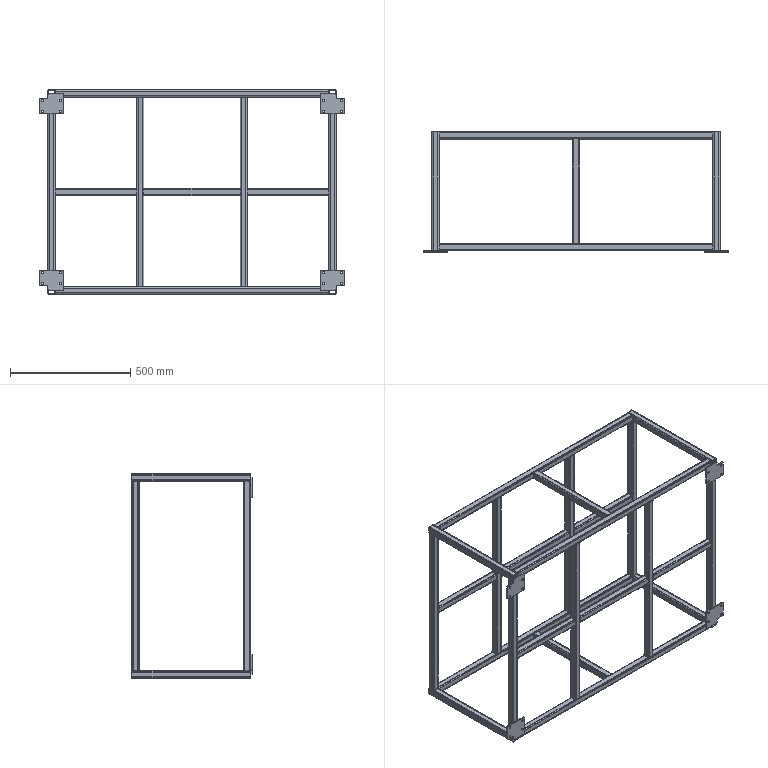Part | SolidWorks | features ReferencePattern 2, AEMSimFeature 1, LocalLPattern 1 | 28 solids | 520 faces | box 1270 x 501 x 850 mm | volume 4402575 mm3 | plane 272 | cylinder 248 | commonest cylinder face diameters 5.2 x96 10.4 x96 9 x32 10 x24